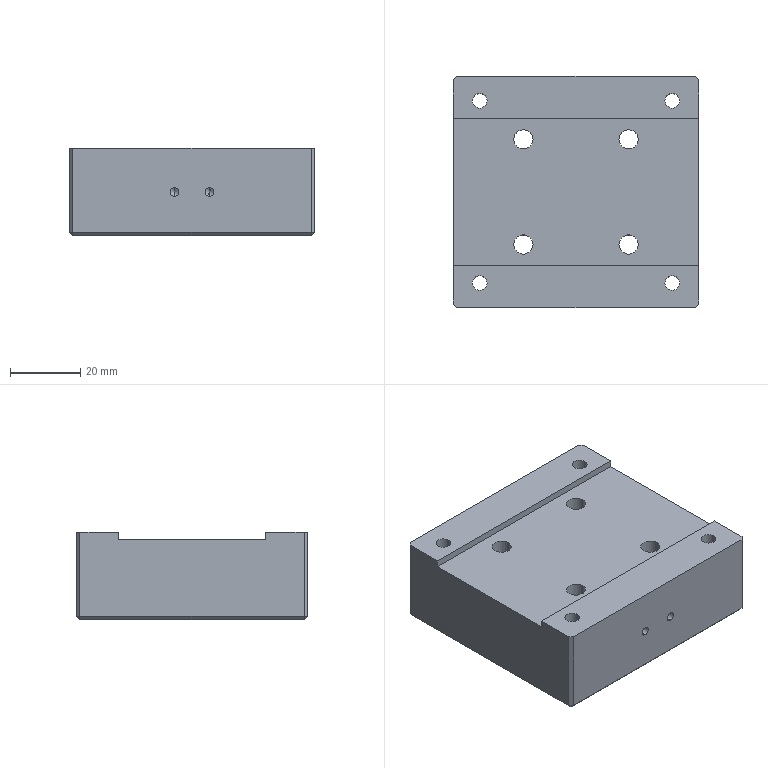Part | STEP file | 10-15 module connection plate | 1 solid | 74 faces | box 70 x 66 x 25 mm | volume 103110 mm3 | cylinder 36 | plane 26 | cone 12 | commonest cylinder face diameters 2.5 x8 4.2 x8 5.5 x8 10 x8 5 x4